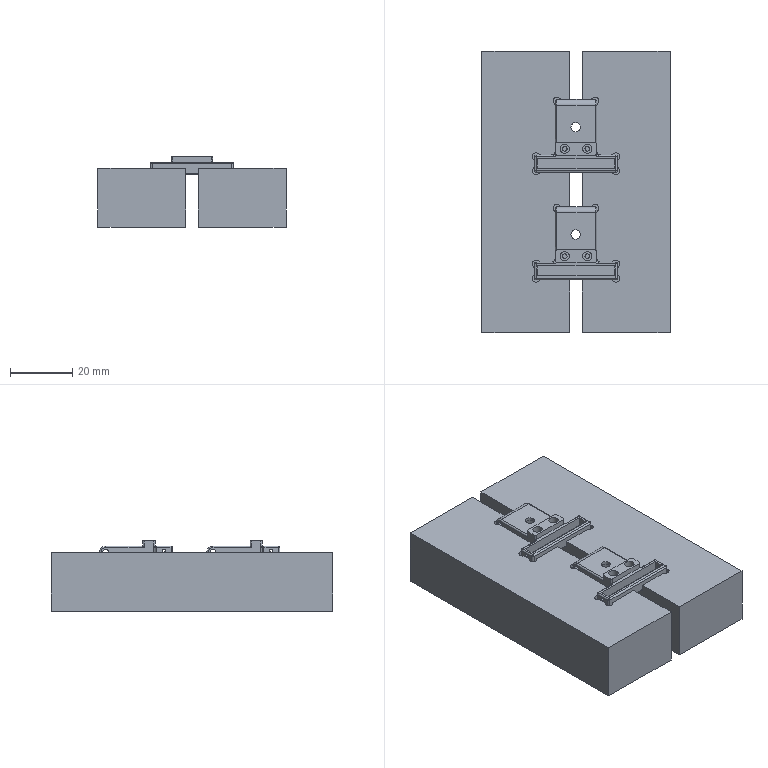Part | 4 solids | 216 faces | box 60.696 x 90.669 x 22.754 mm | volume 98873 mm3 | cylinder 110 | plane 78 | sphere 16 | torus 12 | commonest cylinder face diameters 1 x78 2.5 x12 3 x10 1.5 x4 2 x2 4 x2